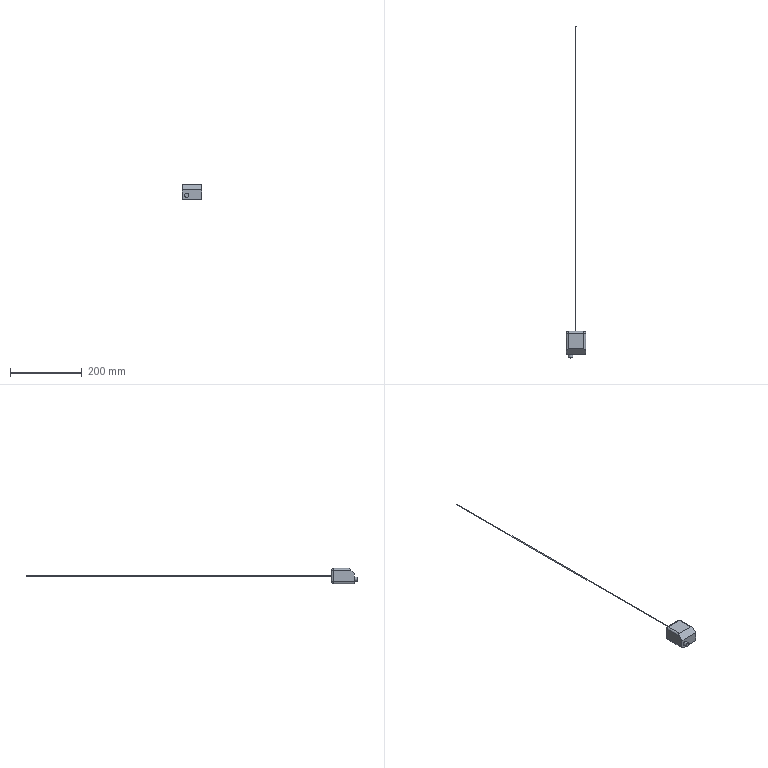Part | NX | 1 solid | 31 faces | box 54 x 924 x 42 mm | volume 140536 mm3 | cylinder 14 | plane 9 | cone 4 | sphere 4 | commonest cylinder face diameters 10 x8 2.5 x4 2 x1 12 x1
STEP:
#1=CARTESIAN_POINT('',(22.,64.,-16.));
#2=VERTEX_POINT('',#1);
#3=CARTESIAN_POINT('',(-22.,64.,-16.));
#4=VERTEX_POINT('',#3);
#5=CARTESIAN_POINT('',(0.,64.,-16.));
#6=DIRECTION('',(-1.,0.,0.));
#7=VECTOR('',#6,1000.);
#8=LINE('',#5,#7);
#9=EDGE_CURVE('',#2,#4,#8,.T.);
#10=ORIENTED_EDGE('',*,*,#9,.T.);
#11=CARTESIAN_POINT('',(-22.,64.,16.));
#12=VERTEX_POINT('',#11);
#13=CARTESIAN_POINT('',(-22.,64.,0.));
#14=DIRECTION('',(0.,0.,1.));
#15=VECTOR('',#14,1000.);
#16=LINE('',#13,#15);
#17=EDGE_CURVE('',#4,#12,#16,.T.);
#18=ORIENTED_EDGE('',*,*,#17,.T.);
#19=CARTESIAN_POINT('',(22.,64.,16.));
#20=VERTEX_POINT('',#19);
#21=CARTESIAN_POINT('',(0.,64.,16.));
#22=DIRECTION('',(1.,0.,0.));
#23=VECTOR('',#22,1000.);
#24=LINE('',#21,#23);
#25=EDGE_CURVE('',#12,#20,#24,.T.);
#26=ORIENTED_EDGE('',*,*,#25,.T.);
#27=CARTESIAN_POINT('',(22.,64.,0.));
#28=DIRECTION('',(0.,0.,-1.));
#29=VECTOR('',#28,1000.);
#30=LINE('',#27,#29);
#31=EDGE_CURVE('',#20,#2,#30,.T.);
#32=ORIENTED_EDGE('',*,*,#31,.T.);
#33=EDGE_LOOP('',(#10,#18,#26,#32));
#34=FACE_BOUND('',#33,.T.);
#35=CARTESIAN_POINT('',(0.,64.,-1.));
#36=VERTEX_POINT('',#35);
#37=CARTESIAN_POINT('',(0.,64.,0.));
#38=DIRECTION('',(0.,-1.,0.));
#39=DIRECTION('',(0.,0.,-1.));
#40=AXIS2_PLACEMENT_3D('',#37,#38,#39);
#41=CIRCLE('',#40,1.);
#42=EDGE_CURVE('',#36,#36,#41,.F.);
#43=ORIENTED_EDGE('',*,*,#42,.F.);
#44=EDGE_LOOP('',(#43));
#45=FACE_BOUND('',#44,.T.);
#46=CARTESIAN_POINT('',(0.,64.,0.));
#47=DIRECTION('',(0.,-1.,0.));
#48=DIRECTION('',(0.,0.,-1.));
#49=AXIS2_PLACEMENT_3D('',#46,#47,#48);
#50=PLANE('',#49);
#51=ADVANCED_FACE('',(#34,#45),#50,.F.);
#52=CARTESIAN_POINT('',(22.,0.,-21.));
#53=VERTEX_POINT('',#52);
#54=CARTESIAN_POINT('',(-22.,0.,-21.));
#55=VERTEX_POINT('',#54);
#56=CARTESIAN_POINT('',(-27.,0.,-21.));
#57=DIRECTION('',(-1.,0.,0.));
#58=VECTOR('',#57,1000.);
#59=LINE('',#56,#58);
#60=EDGE_CURVE('',#53,#55,#59,.T.);
#61=ORIENTED_EDGE('',*,*,#60,.F.);
#62=CARTESIAN_POINT('',(27.,0.,-16.));
#63=VERTEX_POINT('',#62);
#64=CARTESIAN_POINT('',(22.,0.,-16.));
#65=DIRECTION('',(0.,-1.,0.));
#66=DIRECTION('',(0.,0.,-1.));
#67=AXIS2_PLACEMENT_3D('',#64,#65,#66);
#68=CIRCLE('',#67,5.);
#69=EDGE_CURVE('',#53,#63,#68,.T.);
#70=ORIENTED_EDGE('',*,*,#69,.T.);
#71=CARTESIAN_POINT('',(27.,0.,6.));
#72=VERTEX_POINT('',#71);
#73=CARTESIAN_POINT('',(27.,0.,21.));
#74=DIRECTION('',(0.,0.,-1.));
#75=VECTOR('',#74,1000.);
#76=LINE('',#73,#75);
#77=EDGE_CURVE('',#72,#63,#76,.T.);
#78=ORIENTED_EDGE('',*,*,#77,.F.);
#79=CARTESIAN_POINT('',(-27.,0.,6.));
#80=VERTEX_POINT('',#79);
#81=CARTESIAN_POINT('',(-27.,0.,6.));
#82=DIRECTION('',(-1.,0.,0.));
#83=VECTOR('',#82,1000.);
#84=LINE('',#81,#83);
#85=EDGE_CURVE('',#72,#80,#84,.T.);
#86=ORIENTED_EDGE('',*,*,#85,.T.);
#87=CARTESIAN_POINT('',(-27.,0.,-16.));
#88=VERTEX_POINT('',#87);
#89=CARTESIAN_POINT('',(-27.,0.,21.));
#90=DIRECTION('',(0.,0.,1.));
#91=VECTOR('',#90,1000.);
#92=LINE('',#89,#91);
#93=EDGE_CURVE('',#88,#80,#92,.T.);
#94=ORIENTED_EDGE('',*,*,#93,.F.);
#95=CARTESIAN_POINT('',(-22.,0.,-16.));
#96=DIRECTION('',(0.,-1.,0.));
#97=DIRECTION('',(0.,0.,-1.));
#98=AXIS2_PLACEMENT_3D('',#95,#96,#97);
#99=CIRCLE('',#98,5.);
#100=EDGE_CURVE('',#88,#55,#99,.T.);
#101=ORIENTED_EDGE('',*,*,#100,.T.);
#102=EDGE_LOOP('',(#61,#70,#78,#86,#94,#101));
#103=FACE_BOUND('',#102,.T.);
#104=CARTESIAN_POINT('',(-15.,0.,-15.));
#105=VERTEX_POINT('',#104);
#106=CARTESIAN_POINT('',(-15.,0.,-9.));
#107=DIRECTION('',(0.,-1.,0.));
#108=DIRECTION('',(0.,0.,-1.));
#109=AXIS2_PLACEMENT_3D('',#106,#107,#108);
#110=CIRCLE('',#109,6.);
#111=EDGE_CURVE('',#105,#105,#110,.T.);
#112=ORIENTED_EDGE('',*,*,#111,.F.);
#113=EDGE_LOOP('',(#112));
#114=FACE_BOUND('',#113,.T.);
#115=CARTESIAN_POINT('',(0.,0.,0.));
#116=DIRECTION('',(0.,-1.,0.));
#117=DIRECTION('',(0.,0.,-1.));
#118=AXIS2_PLACEMENT_3D('',#115,#116,#117);
#119=PLANE('',#118);
#120=ADVANCED_FACE('',(#103,#114),#119,.T.);
#121=CARTESIAN_POINT('',(27.,59.,-16.));
#122=VERTEX_POINT('',#121);
#123=CARTESIAN_POINT('',(27.,64.,-16.));
#124=DIRECTION('',(0.,-1.,0.));
#125=VECTOR('',#124,1000.);
#126=LINE('',#123,#125);
#127=EDGE_CURVE('',#63,#122,#126,.F.);
#128=ORIENTED_EDGE('',*,*,#127,.T.);
#129=CARTESIAN_POINT('',(27.,59.,16.));
#130=VERTEX_POINT('',#129);
#131=CARTESIAN_POINT('',(27.,59.,21.));
#132=DIRECTION('',(0.,0.,-1.));
#133=VECTOR('',#132,1000.);
#134=LINE('',#131,#133);
#135=EDGE_CURVE('',#122,#130,#134,.F.);
#136=ORIENTED_EDGE('',*,*,#135,.T.);
#137=CARTESIAN_POINT('',(27.,10.,16.));
#138=VERTEX_POINT('',#137);
#139=CARTESIAN_POINT('',(27.,64.,16.));
#140=DIRECTION('',(0.,-1.,0.));
#141=VECTOR('',#140,1000.);
#142=LINE('',#139,#141);
#143=EDGE_CURVE('',#130,#138,#142,.T.);
#144=ORIENTED_EDGE('',*,*,#143,.T.);
#145=CARTESIAN_POINT('',(27.,15.,21.));
#146=DIRECTION('',(0.,-0.7071,-0.7071));
#147=VECTOR('',#146,1000.);
#148=LINE('',#145,#147);
#149=EDGE_CURVE('',#138,#72,#148,.T.);
#150=ORIENTED_EDGE('',*,*,#149,.T.);
#151=ORIENTED_EDGE('',*,*,#77,.T.);
#152=EDGE_LOOP('',(#128,#136,#144,#150,#151));
#153=FACE_BOUND('',#152,.T.);
#154=CARTESIAN_POINT('',(27.,64.,21.));
#155=DIRECTION('',(-1.,0.,0.));
#156=DIRECTION('',(0.,0.,1.));
#157=AXIS2_PLACEMENT_3D('',#154,#155,#156);
#158=PLANE('',#157);
#159=ADVANCED_FACE('',(#153),#158,.F.);
#160=CARTESIAN_POINT('',(17.25,46.4,-21.));
#161=VERTEX_POINT('',#160);
#162=CARTESIAN_POINT('',(18.5,46.4,-21.));
#163=DIRECTION('',(0.,0.,-1.));
#164=DIRECTION('',(-1.,0.,0.));
#165=AXIS2_PLACEMENT_3D('',#162,#163,#164);
#166=CIRCLE('',#165,1.25);
#167=EDGE_CURVE('',#161,#161,#166,.T.);
#168=ORIENTED_EDGE('',*,*,#167,.F.);
#169=EDGE_LOOP('',(#168));
#170=FACE_BOUND('',#169,.T.);
#171=CARTESIAN_POINT('',(-19.75,46.4,-21.));
#172=VERTEX_POINT('',#171);
#173=CARTESIAN_POINT('',(-18.5,46.4,-21.));
#174=DIRECTION('',(0.,0.,-1.));
#175=DIRECTION('',(-1.,0.,0.));
#176=AXIS2_PLACEMENT_3D('',#173,#174,#175);
#177=CIRCLE('',#176,1.25);
#178=EDGE_CURVE('',#172,#172,#177,.T.);
#179=ORIENTED_EDGE('',*,*,#178,.F.);
#180=EDGE_LOOP('',(#179));
#181=FACE_BOUND('',#180,.T.);
#182=CARTESIAN_POINT('',(17.25,26.4,-21.));
#183=VERTEX_POINT('',#182);
#184=CARTESIAN_POINT('',(18.5,26.4,-21.));
#185=DIRECTION('',(0.,0.,-1.));
#186=DIRECTION('',(-1.,0.,0.));
#187=AXIS2_PLACEMENT_3D('',#184,#185,#186);
#188=CIRCLE('',#187,1.25);
#189=EDGE_CURVE('',#183,#183,#188,.T.);
#190=ORIENTED_EDGE('',*,*,#189,.F.);
#191=EDGE_LOOP('',(#190));
#192=FACE_BOUND('',#191,.T.);
#193=CARTESIAN_POINT('',(-19.75,26.4,-21.));
#194=VERTEX_POINT('',#193);
#195=CARTESIAN_POINT('',(-18.5,26.4,-21.));
#196=DIRECTION('',(0.,0.,-1.));
#197=DIRECTION('',(-1.,0.,0.));
#198=AXIS2_PLACEMENT_3D('',#195,#196,#197);
#199=CIRCLE('',#198,1.25);
#200=EDGE_CURVE('',#194,#194,#199,.T.);
#201=ORIENTED_EDGE('',*,*,#200,.F.);
#202=EDGE_LOOP('',(#201));
#203=FACE_BOUND('',#202,.T.);
#204=CARTESIAN_POINT('',(-22.,59.,-21.));
#205=VERTEX_POINT('',#204);
#206=CARTESIAN_POINT('',(-22.,64.,-21.));
#207=DIRECTION('',(0.,-1.,0.));
#208=VECTOR('',#207,1000.);
#209=LINE('',#206,#208);
#210=EDGE_CURVE('',#55,#205,#209,.F.);
#211=ORIENTED_EDGE('',*,*,#210,.T.);
#212=CARTESIAN_POINT('',(22.,59.,-21.));
#213=VERTEX_POINT('',#212);
#214=CARTESIAN_POINT('',(-27.,59.,-21.));
#215=DIRECTION('',(-1.,0.,0.));
#216=VECTOR('',#215,1000.);
#217=LINE('',#214,#216);
#218=EDGE_CURVE('',#205,#213,#217,.F.);
#219=ORIENTED_EDGE('',*,*,#218,.T.);
#220=CARTESIAN_POINT('',(22.,64.,-21.));
#221=DIRECTION('',(0.,-1.,0.));
#222=VECTOR('',#221,1000.);
#223=LINE('',#220,#222);
#224=EDGE_CURVE('',#213,#53,#223,.T.);
#225=ORIENTED_EDGE('',*,*,#224,.T.);
#226=ORIENTED_EDGE('',*,*,#60,.T.);
#227=EDGE_LOOP('',(#211,#219,#225,#226));
#228=FACE_BOUND('',#227,.T.);
#229=CARTESIAN_POINT('',(-27.,64.,-21.));
#230=DIRECTION('',(0.,0.,1.));
#231=DIRECTION('',(1.,0.,0.));
#232=AXIS2_PLACEMENT_3D('',#229,#230,#231);
#233=PLANE('',#232);
#234=ADVANCED_FACE('',(#170,#181,#192,#203,#228),#233,.F.);
#235=CARTESIAN_POINT('',(-27.,10.,16.));
#236=VERTEX_POINT('',#235);
#237=CARTESIAN_POINT('',(-27.,59.,16.));
#238=VERTEX_POINT('',#237);
#239=CARTESIAN_POINT('',(-27.,64.,16.));
#240=DIRECTION('',(0.,-1.,0.));
#241=VECTOR('',#240,1000.);
#242=LINE('',#239,#241);
#243=EDGE_CURVE('',#236,#238,#242,.F.);
#244=ORIENTED_EDGE('',*,*,#243,.T.);
#245=CARTESIAN_POINT('',(-27.,59.,-16.));
#246=VERTEX_POINT('',#245);
#247=CARTESIAN_POINT('',(-27.,59.,21.));
#248=DIRECTION('',(0.,0.,1.));
#249=VECTOR('',#248,1000.);
#250=LINE('',#247,#249);
#251=EDGE_CURVE('',#238,#246,#250,.F.);
#252=ORIENTED_EDGE('',*,*,#251,.T.);
#253=CARTESIAN_POINT('',(-27.,64.,-16.));
#254=DIRECTION('',(0.,-1.,0.));
#255=VECTOR('',#254,1000.);
#256=LINE('',#253,#255);
#257=EDGE_CURVE('',#246,#88,#256,.T.);
#258=ORIENTED_EDGE('',*,*,#257,.T.);
#259=ORIENTED_EDGE('',*,*,#93,.T.);
#260=CARTESIAN_POINT('',(-27.,15.,21.));
#261=DIRECTION('',(0.,0.7071,0.7071));
#262=VECTOR('',#261,1000.);
#263=LINE('',#260,#262);
#264=EDGE_CURVE('',#80,#236,#263,.T.);
#265=ORIENTED_EDGE('',*,*,#264,.T.);
#266=EDGE_LOOP('',(#244,#252,#258,#259,#265));
#267=FACE_BOUND('',#266,.T.);
#268=CARTESIAN_POINT('',(-27.,64.,21.));
#269=DIRECTION('',(1.,0.,0.));
#270=DIRECTION('',(0.,0.,-1.));
#271=AXIS2_PLACEMENT_3D('',#268,#269,#270);
#272=PLANE('',#271);
#273=ADVANCED_FACE('',(#267),#272,.F.);
#274=CARTESIAN_POINT('',(22.,15.,21.));
#275=VERTEX_POINT('',#274);
#276=CARTESIAN_POINT('',(22.,59.,21.));
#277=VERTEX_POINT('',#276);
#278=CARTESIAN_POINT('',(22.,64.,21.));
#279=DIRECTION('',(0.,-1.,0.));
#280=VECTOR('',#279,1000.);
#281=LINE('',#278,#280);
#282=EDGE_CURVE('',#275,#277,#281,.F.);
#283=ORIENTED_EDGE('',*,*,#282,.T.);
#284=CARTESIAN_POINT('',(-22.,59.,21.));
#285=VERTEX_POINT('',#284);
#286=CARTESIAN_POINT('',(-27.,59.,21.));
#287=DIRECTION('',(1.,0.,0.));
#288=VECTOR('',#287,1000.);
#289=LINE('',#286,#288);
#290=EDGE_CURVE('',#277,#285,#289,.F.);
#291=ORIENTED_EDGE('',*,*,#290,.T.);
#292=CARTESIAN_POINT('',(-22.,15.,21.));
#293=VERTEX_POINT('',#292);
#294=CARTESIAN_POINT('',(-22.,64.,21.));
#295=DIRECTION('',(0.,-1.,0.));
#296=VECTOR('',#295,1000.);
#297=LINE('',#294,#296);
#298=EDGE_CURVE('',#285,#293,#297,.T.);
#299=ORIENTED_EDGE('',*,*,#298,.T.);
#300=CARTESIAN_POINT('',(27.,15.,21.));
#301=DIRECTION('',(1.,0.,0.));
#302=VECTOR('',#301,1000.);
#303=LINE('',#300,#302);
#304=EDGE_CURVE('',#293,#275,#303,.T.);
#305=ORIENTED_EDGE('',*,*,#304,.T.);
#306=EDGE_LOOP('',(#283,#291,#299,#305));
#307=FACE_BOUND('',#306,.T.);
#308=CARTESIAN_POINT('',(-27.,64.,21.));
#309=DIRECTION('',(0.,0.,-1.));
#310=DIRECTION('',(-1.,0.,0.));
#311=AXIS2_PLACEMENT_3D('',#308,#309,#310);
#312=PLANE('',#311);
#313=ADVANCED_FACE('',(#307),#312,.F.);
#314=ORIENTED_EDGE('',*,*,#149,.F.);
#315=CARTESIAN_POINT('',(22.,10.,16.));
#316=DIRECTION('',(0.,-0.7071,0.7071));
#317=DIRECTION('',(0.,-0.7071,-0.7071));
#318=AXIS2_PLACEMENT_3D('',#315,#316,#317);
#319=ELLIPSE('',#318,7.071,5.);
#320=EDGE_CURVE('',#138,#275,#319,.T.);
#321=ORIENTED_EDGE('',*,*,#320,.T.);
#322=ORIENTED_EDGE('',*,*,#304,.F.);
#323=CARTESIAN_POINT('',(-22.,10.,16.));
#324=DIRECTION('',(0.,-0.7071,0.7071));
#325=DIRECTION('',(0.,-0.7071,-0.7071));
#326=AXIS2_PLACEMENT_3D('',#323,#324,#325);
#327=ELLIPSE('',#326,7.071,5.);
#328=EDGE_CURVE('',#293,#236,#327,.T.);
#329=ORIENTED_EDGE('',*,*,#328,.T.);
#330=ORIENTED_EDGE('',*,*,#264,.F.);
#331=ORIENTED_EDGE('',*,*,#85,.F.);
#332=EDGE_LOOP('',(#314,#321,#322,#329,#330,#331));
#333=FACE_BOUND('',#332,.T.);
#334=CARTESIAN_POINT('',(-27.,15.,21.));
#335=DIRECTION('',(0.,-0.7071,0.7071));
#336=DIRECTION('',(-1.,0.,0.));
#337=AXIS2_PLACEMENT_3D('',#334,#335,#336);
#338=PLANE('',#337);
#339=ADVANCED_FACE('',(#333),#338,.T.);
#340=CARTESIAN_POINT('',(-18.5,26.4,-11.749));
#341=VERTEX_POINT('',#340);
#342=VERTEX_LOOP('',#341);
#343=FACE_BOUND('',#342,.T.);
#344=CARTESIAN_POINT('',(-19.75,26.4,-12.5));
#345=VERTEX_POINT('',#344);
#346=CARTESIAN_POINT('',(-18.5,26.4,-12.5));
#347=DIRECTION('',(0.,0.,-1.));
#348=DIRECTION('',(-1.,0.,0.));
#349=AXIS2_PLACEMENT_3D('',#346,#347,#348);
#350=CIRCLE('',#349,1.25);
#351=EDGE_CURVE('',#345,#345,#350,.T.);
#352=ORIENTED_EDGE('',*,*,#351,.T.);
#353=EDGE_LOOP('',(#352));
#354=FACE_BOUND('',#353,.T.);
#355=CARTESIAN_POINT('',(-18.5,26.4,-12.5));
#356=DIRECTION('',(0.,0.,-1.));
#357=DIRECTION('',(-1.,0.,0.));
#358=AXIS2_PLACEMENT_3D('',#355,#356,#357);
#359=CONICAL_SURFACE('',#358,1.25,1.03);
#360=ADVANCED_FACE('',(#343,#354),#359,.F.);
#361=ORIENTED_EDGE('',*,*,#351,.F.);
#362=EDGE_LOOP('',(#361));
#363=FACE_BOUND('',#362,.T.);
#364=ORIENTED_EDGE('',*,*,#200,.T.);
#365=EDGE_LOOP('',(#364));
#366=FACE_BOUND('',#365,.T.);
#367=CARTESIAN_POINT('',(-18.5,26.4,-21.));
#368=DIRECTION('',(0.,0.,-1.));
#369=DIRECTION('',(-1.,0.,0.));
#370=AXIS2_PLACEMENT_3D('',#367,#368,#369);
#371=CYLINDRICAL_SURFACE('',#370,1.25);
#372=ADVANCED_FACE('',(#363,#366),#371,.F.);
#373=CARTESIAN_POINT('',(18.5,26.4,-11.749));
#374=VERTEX_POINT('',#373);
#375=VERTEX_LOOP('',#374);
#376=FACE_BOUND('',#375,.T.);
#377=CARTESIAN_POINT('',(17.25,26.4,-12.5));
#378=VERTEX_POINT('',#377);
#379=CARTESIAN_POINT('',(18.5,26.4,-12.5));
#380=DIRECTION('',(0.,0.,-1.));
#381=DIRECTION('',(-1.,0.,0.));
#382=AXIS2_PLACEMENT_3D('',#379,#380,#381);
#383=CIRCLE('',#382,1.25);
#384=EDGE_CURVE('',#378,#378,#383,.T.);
#385=ORIENTED_EDGE('',*,*,#384,.T.);
#386=EDGE_LOOP('',(#385));
#387=FACE_BOUND('',#386,.T.);
#388=CARTESIAN_POINT('',(18.5,26.4,-12.5));
#389=DIRECTION('',(0.,0.,-1.));
#390=DIRECTION('',(-1.,0.,0.));
#391=AXIS2_PLACEMENT_3D('',#388,#389,#390);
#392=CONICAL_SURFACE('',#391,1.25,1.03);
#393=ADVANCED_FACE('',(#376,#387),#392,.F.);
#394=ORIENTED_EDGE('',*,*,#384,.F.);
#395=EDGE_LOOP('',(#394));
#396=FACE_BOUND('',#395,.T.);
#397=ORIENTED_EDGE('',*,*,#189,.T.);
#398=EDGE_LOOP('',(#397));
#399=FACE_BOUND('',#398,.T.);
#400=CARTESIAN_POINT('',(18.5,26.4,-21.));
#401=DIRECTION('',(0.,0.,-1.));
#402=DIRECTION('',(-1.,0.,0.));
#403=AXIS2_PLACEMENT_3D('',#400,#401,#402);
#404=CYLINDRICAL_SURFACE('',#403,1.25);
#405=ADVANCED_FACE('',(#396,#399),#404,.F.);
#406=CARTESIAN_POINT('',(-18.5,46.4,-11.749));
#407=VERTEX_POINT('',#406);
#408=VERTEX_LOOP('',#407);
#409=FACE_BOUND('',#408,.T.);
#410=CARTESIAN_POINT('',(-19.75,46.4,-12.5));
#411=VERTEX_POINT('',#410);
#412=CARTESIAN_POINT('',(-18.5,46.4,-12.5));
#413=DIRECTION('',(0.,0.,-1.));
#414=DIRECTION('',(-1.,0.,0.));
#415=AXIS2_PLACEMENT_3D('',#412,#413,#414);
#416=CIRCLE('',#415,1.25);
#417=EDGE_CURVE('',#411,#411,#416,.T.);
#418=ORIENTED_EDGE('',*,*,#417,.T.);
#419=EDGE_LOOP('',(#418));
#420=FACE_BOUND('',#419,.T.);
#421=CARTESIAN_POINT('',(-18.5,46.4,-12.5));
#422=DIRECTION('',(0.,0.,-1.));
#423=DIRECTION('',(-1.,0.,0.));
#424=AXIS2_PLACEMENT_3D('',#421,#422,#423);
#425=CONICAL_SURFACE('',#424,1.25,1.03);
#426=ADVANCED_FACE('',(#409,#420),#425,.F.);
#427=ORIENTED_EDGE('',*,*,#417,.F.);
#428=EDGE_LOOP('',(#427));
#429=FACE_BOUND('',#428,.T.);
#430=ORIENTED_EDGE('',*,*,#178,.T.);
#431=EDGE_LOOP('',(#430));
#432=FACE_BOUND('',#431,.T.);
#433=CARTESIAN_POINT('',(-18.5,46.4,-21.));
#434=DIRECTION('',(0.,0.,-1.));
#435=DIRECTION('',(-1.,0.,0.));
#436=AXIS2_PLACEMENT_3D('',#433,#434,#435);
#437=CYLINDRICAL_SURFACE('',#436,1.25);
#438=ADVANCED_FACE('',(#429,#432),#437,.F.);
#439=CARTESIAN_POINT('',(18.5,46.4,-11.749));
#440=VERTEX_POINT('',#439);
#441=VERTEX_LOOP('',#440);
#442=FACE_BOUND('',#441,.T.);
#443=CARTESIAN_POINT('',(17.25,46.4,-12.5));
#444=VERTEX_POINT('',#443);
#445=CARTESIAN_POINT('',(18.5,46.4,-12.5));
#446=DIRECTION('',(0.,0.,-1.));
#447=DIRECTION('',(-1.,0.,0.));
#448=AXIS2_PLACEMENT_3D('',#445,#446,#447);
#449=CIRCLE('',#448,1.25);
#450=EDGE_CURVE('',#444,#444,#449,.T.);
#451=ORIENTED_EDGE('',*,*,#450,.T.);
#452=EDGE_LOOP('',(#451));
#453=FACE_BOUND('',#452,.T.);
#454=CARTESIAN_POINT('',(18.5,46.4,-12.5));
#455=DIRECTION('',(0.,0.,-1.));
#456=DIRECTION('',(-1.,0.,0.));
#457=AXIS2_PLACEMENT_3D('',#454,#455,#456);
#458=CONICAL_SURFACE('',#457,1.25,1.03);
#459=ADVANCED_FACE('',(#442,#453),#458,.F.);
#460=ORIENTED_EDGE('',*,*,#450,.F.);
#461=EDGE_LOOP('',(#460));
#462=FACE_BOUND('',#461,.T.);
#463=ORIENTED_EDGE('',*,*,#167,.T.);
#464=EDGE_LOOP('',(#463));
#465=FACE_BOUND('',#464,.T.);
#466=CARTESIAN_POINT('',(18.5,46.4,-21.));
#467=DIRECTION('',(0.,0.,-1.));
#468=DIRECTION('',(-1.,0.,0.));
#469=AXIS2_PLACEMENT_3D('',#466,#467,#468);
#470=CYLINDRICAL_SURFACE('',#469,1.25);
#471=ADVANCED_FACE('',(#462,#465),#470,.F.);
#472=ORIENTED_EDGE('',*,*,#143,.F.);
#473=CARTESIAN_POINT('',(22.,59.,16.));
#474=DIRECTION('',(0.,-1.,0.));
#475=DIRECTION('',(0.,0.,-1.));
#476=AXIS2_PLACEMENT_3D('',#473,#474,#475);
#477=CIRCLE('',#476,5.);
#478=EDGE_CURVE('',#130,#277,#477,.T.);
#479=ORIENTED_EDGE('',*,*,#478,.T.);
#480=ORIENTED_EDGE('',*,*,#282,.F.);
#481=ORIENTED_EDGE('',*,*,#320,.F.);
#482=EDGE_LOOP('',(#472,#479,#480,#481));
#483=FACE_BOUND('',#482,.T.);
#484=CARTESIAN_POINT('',(22.,64.,16.));
#485=DIRECTION('',(0.,-1.,0.));
#486=DIRECTION('',(0.,0.,-1.));
#487=AXIS2_PLACEMENT_3D('',#484,#485,#486);
#488=CYLINDRICAL_SURFACE('',#487,5.);
#489=ADVANCED_FACE('',(#483),#488,.T.);
#490=ORIENTED_EDGE('',*,*,#298,.F.);
#491=CARTESIAN_POINT('',(-22.,59.,16.));
#492=DIRECTION('',(0.,-1.,0.));
#493=DIRECTION('',(0.,0.,-1.));
#494=AXIS2_PLACEMENT_3D('',#491,#492,#493);
#495=CIRCLE('',#494,5.);
#496=EDGE_CURVE('',#285,#238,#495,.T.);
#497=ORIENTED_EDGE('',*,*,#496,.T.);
#498=ORIENTED_EDGE('',*,*,#243,.F.);
#499=ORIENTED_EDGE('',*,*,#328,.F.);
#500=EDGE_LOOP('',(#490,#497,#498,#499));
#501=FACE_BOUND('',#500,.T.);
#502=CARTESIAN_POINT('',(-22.,64.,16.));
#503=DIRECTION('',(0.,-1.,0.));
#504=DIRECTION('',(0.,0.,-1.));
#505=AXIS2_PLACEMENT_3D('',#502,#503,#504);
#506=CYLINDRICAL_SURFACE('',#505,5.);
#507=ADVANCED_FACE('',(#501),#506,.T.);
#508=ORIENTED_EDGE('',*,*,#224,.F.);
#509=CARTESIAN_POINT('',(22.,59.,-16.));
#510=DIRECTION('',(0.,-1.,0.));
#511=DIRECTION('',(0.,0.,-1.));
#512=AXIS2_PLACEMENT_3D('',#509,#510,#511);
#513=CIRCLE('',#512,5.);
#514=EDGE_CURVE('',#213,#122,#513,.T.);
#515=ORIENTED_EDGE('',*,*,#514,.T.);
#516=ORIENTED_EDGE('',*,*,#127,.F.);
#517=ORIENTED_EDGE('',*,*,#69,.F.);
#518=EDGE_LOOP('',(#508,#515,#516,#517));
#519=FACE_BOUND('',#518,.T.);
#520=CARTESIAN_POINT('',(22.,64.,-16.));
#521=DIRECTION('',(0.,-1.,0.));
#522=DIRECTION('',(0.,0.,-1.));
#523=AXIS2_PLACEMENT_3D('',#520,#521,#522);
#524=CYLINDRICAL_SURFACE('',#523,5.);
#525=ADVANCED_FACE('',(#519),#524,.T.);
#526=ORIENTED_EDGE('',*,*,#257,.F.);
#527=CARTESIAN_POINT('',(-22.,59.,-16.));
#528=DIRECTION('',(0.,-1.,0.));
#529=DIRECTION('',(0.,0.,-1.));
#530=AXIS2_PLACEMENT_3D('',#527,#528,#529);
#531=CIRCLE('',#530,5.);
#532=EDGE_CURVE('',#246,#205,#531,.T.);
#533=ORIENTED_EDGE('',*,*,#532,.T.);
#534=ORIENTED_EDGE('',*,*,#210,.F.);
#535=ORIENTED_EDGE('',*,*,#100,.F.);
#536=EDGE_LOOP('',(#526,#533,#534,#535));
#537=FACE_BOUND('',#536,.T.);
#538=CARTESIAN_POINT('',(-22.,64.,-16.));
#539=DIRECTION('',(0.,-1.,0.));
#540=DIRECTION('',(0.,0.,-1.));
#541=AXIS2_PLACEMENT_3D('',#538,#539,#540);
#542=CYLINDRICAL_SURFACE('',#541,5.);
#543=ADVANCED_FACE('',(#537),#542,.T.);
#544=CARTESIAN_POINT('',(-15.,-10.,-15.));
#545=VERTEX_POINT('',#544);
#546=CARTESIAN_POINT('',(-15.,-10.,-9.));
#547=DIRECTION('',(0.,-1.,0.));
#548=DIRECTION('',(0.,0.,-1.));
#549=AXIS2_PLACEMENT_3D('',#546,#547,#548);
#550=CIRCLE('',#549,6.);
#551=EDGE_CURVE('',#545,#545,#550,.T.);
#552=ORIENTED_EDGE('',*,*,#551,.F.);
#553=EDGE_LOOP('',(#552));
#554=FACE_BOUND('',#553,.T.);
#555=ORIENTED_EDGE('',*,*,#111,.T.);
#556=EDGE_LOOP('',(#555));
#557=FACE_BOUND('',#556,.T.);
#558=CARTESIAN_POINT('',(-15.,-10.,-9.));
#559=DIRECTION('',(0.,1.,0.));
#560=DIRECTION('',(0.,0.,1.));
#561=AXIS2_PLACEMENT_3D('',#558,#559,#560);
#562=CYLINDRICAL_SURFACE('',#561,6.);
#563=ADVANCED_FACE('',(#554,#557),#562,.T.);
#564=ORIENTED_EDGE('',*,*,#551,.T.);
#565=EDGE_LOOP('',(#564));
#566=FACE_BOUND('',#565,.T.);
#567=CARTESIAN_POINT('',(-15.,-10.,-9.));
#568=DIRECTION('',(0.,-1.,0.));
#569=DIRECTION('',(0.,0.,-1.));
#570=AXIS2_PLACEMENT_3D('',#567,#568,#569);
#571=PLANE('',#570);
#572=ADVANCED_FACE('',(#566),#571,.T.);
#573=CARTESIAN_POINT('',(22.,59.,-16.));
#574=DIRECTION('',(0.,0.,1.));
#575=DIRECTION('',(1.,0.,0.));
#576=AXIS2_PLACEMENT_3D('',#573,#574,#575);
#577=CIRCLE('',#576,5.);
#578=EDGE_CURVE('',#122,#2,#577,.T.);
#579=ORIENTED_EDGE('',*,*,#578,.F.);
#580=ORIENTED_EDGE('',*,*,#514,.F.);
#581=CARTESIAN_POINT('',(22.,59.,-16.));
#582=DIRECTION('',(-1.,0.,0.));
#583=DIRECTION('',(0.,0.,1.));
#584=AXIS2_PLACEMENT_3D('',#581,#582,#583);
#585=CIRCLE('',#584,5.);
#586=EDGE_CURVE('',#2,#213,#585,.T.);
#587=ORIENTED_EDGE('',*,*,#586,.F.);
#588=EDGE_LOOP('',(#579,#580,#587));
#589=FACE_BOUND('',#588,.T.);
#590=CARTESIAN_POINT('',(22.,59.,-16.));
#591=DIRECTION('',(0.,0.,1.));
#592=DIRECTION('',(1.,0.,0.));
#593=AXIS2_PLACEMENT_3D('',#590,#591,#592);
#594=SPHERICAL_SURFACE('',#593,5.);
#595=ADVANCED_FACE('',(#589),#594,.T.);
#596=ORIENTED_EDGE('',*,*,#586,.T.);
#597=ORIENTED_EDGE('',*,*,#218,.F.);
#598=CARTESIAN_POINT('',(-22.,59.,-16.));
#599=DIRECTION('',(-1.,0.,0.));
#600=DIRECTION('',(0.,0.,1.));
#601=AXIS2_PLACEMENT_3D('',#598,#599,#600);
#602=CIRCLE('',#601,5.);
#603=EDGE_CURVE('',#4,#205,#602,.T.);
#604=ORIENTED_EDGE('',*,*,#603,.F.);
#605=ORIENTED_EDGE('',*,*,#9,.F.);
#606=EDGE_LOOP('',(#596,#597,#604,#605));
#607=FACE_BOUND('',#606,.T.);
#608=CARTESIAN_POINT('',(0.,59.,-16.));
#609=DIRECTION('',(-1.,0.,0.));
#610=DIRECTION('',(0.,0.,1.));
#611=AXIS2_PLACEMENT_3D('',#608,#609,#610);
#612=CYLINDRICAL_SURFACE('',#611,5.);
#613=ADVANCED_FACE('',(#607),#612,.T.);
#614=ORIENTED_EDGE('',*,*,#578,.T.);
#615=ORIENTED_EDGE('',*,*,#31,.F.);
#616=CARTESIAN_POINT('',(22.,59.,16.));
#617=DIRECTION('',(0.,0.,1.));
#618=DIRECTION('',(1.,0.,0.));
#619=AXIS2_PLACEMENT_3D('',#616,#617,#618);
#620=CIRCLE('',#619,5.);
#621=EDGE_CURVE('',#130,#20,#620,.T.);
#622=ORIENTED_EDGE('',*,*,#621,.F.);
#623=ORIENTED_EDGE('',*,*,#135,.F.);
#624=EDGE_LOOP('',(#614,#615,#622,#623));
#625=FACE_BOUND('',#624,.T.);
#626=CARTESIAN_POINT('',(22.,59.,0.));
#627=DIRECTION('',(0.,0.,-1.));
#628=DIRECTION('',(-1.,0.,0.));
#629=AXIS2_PLACEMENT_3D('',#626,#627,#628);
#630=CYLINDRICAL_SURFACE('',#629,5.);
#631=ADVANCED_FACE('',(#625),#630,.T.);
#632=ORIENTED_EDGE('',*,*,#603,.T.);
#633=ORIENTED_EDGE('',*,*,#532,.F.);
#634=CARTESIAN_POINT('',(-22.,59.,-16.));
#635=DIRECTION('',(0.,0.,1.));
#636=DIRECTION('',(1.,0.,0.));
#637=AXIS2_PLACEMENT_3D('',#634,#635,#636);
#638=CIRCLE('',#637,5.);
#639=EDGE_CURVE('',#4,#246,#638,.T.);
#640=ORIENTED_EDGE('',*,*,#639,.F.);
#641=EDGE_LOOP('',(#632,#633,#640));
#642=FACE_BOUND('',#641,.T.);
#643=CARTESIAN_POINT('',(-22.,59.,-16.));
#644=DIRECTION('',(0.,0.,1.));
#645=DIRECTION('',(1.,0.,0.));
#646=AXIS2_PLACEMENT_3D('',#643,#644,#645);
#647=SPHERICAL_SURFACE('',#646,5.);
#648=ADVANCED_FACE('',(#642),#647,.T.);
#649=ORIENTED_EDGE('',*,*,#478,.F.);
#650=ORIENTED_EDGE('',*,*,#621,.T.);
#651=CARTESIAN_POINT('',(22.,59.,16.));
#652=DIRECTION('',(-1.,0.,0.));
#653=DIRECTION('',(0.,0.,1.));
#654=AXIS2_PLACEMENT_3D('',#651,#652,#653);
#655=CIRCLE('',#654,5.);
#656=EDGE_CURVE('',#277,#20,#655,.T.);
#657=ORIENTED_EDGE('',*,*,#656,.F.);
#658=EDGE_LOOP('',(#649,#650,#657));
#659=FACE_BOUND('',#658,.T.);
#660=CARTESIAN_POINT('',(22.,59.,16.));
#661=DIRECTION('',(0.,0.,1.));
#662=DIRECTION('',(1.,0.,0.));
#663=AXIS2_PLACEMENT_3D('',#660,#661,#662);
#664=SPHERICAL_SURFACE('',#663,5.);
#665=ADVANCED_FACE('',(#659),#664,.T.);
#666=ORIENTED_EDGE('',*,*,#639,.T.);
#667=ORIENTED_EDGE('',*,*,#251,.F.);
#668=CARTESIAN_POINT('',(-22.,59.,16.));
#669=DIRECTION('',(0.,0.,1.));
#670=DIRECTION('',(1.,0.,0.));
#671=AXIS2_PLACEMENT_3D('',#668,#669,#670);
#672=CIRCLE('',#671,5.);
#673=EDGE_CURVE('',#12,#238,#672,.T.);
#674=ORIENTED_EDGE('',*,*,#673,.F.);
#675=ORIENTED_EDGE('',*,*,#17,.F.);
#676=EDGE_LOOP('',(#666,#667,#674,#675));
#677=FACE_BOUND('',#676,.T.);
#678=CARTESIAN_POINT('',(-22.,59.,0.));
#679=DIRECTION('',(0.,0.,1.));
#680=DIRECTION('',(1.,0.,0.));
#681=AXIS2_PLACEMENT_3D('',#678,#679,#680);
#682=CYLINDRICAL_SURFACE('',#681,5.);
#683=ADVANCED_FACE('',(#677),#682,.T.);
#684=ORIENTED_EDGE('',*,*,#656,.T.);
#685=ORIENTED_EDGE('',*,*,#25,.F.);
#686=CARTESIAN_POINT('',(-22.,59.,16.));
#687=DIRECTION('',(-1.,0.,0.));
#688=DIRECTION('',(0.,0.,1.));
#689=AXIS2_PLACEMENT_3D('',#686,#687,#688);
#690=CIRCLE('',#689,5.);
#691=EDGE_CURVE('',#285,#12,#690,.T.);
#692=ORIENTED_EDGE('',*,*,#691,.F.);
#693=ORIENTED_EDGE('',*,*,#290,.F.);
#694=EDGE_LOOP('',(#684,#685,#692,#693));
#695=FACE_BOUND('',#694,.T.);
#696=CARTESIAN_POINT('',(0.,59.,16.));
#697=DIRECTION('',(1.,0.,0.));
#698=DIRECTION('',(0.,0.,-1.));
#699=AXIS2_PLACEMENT_3D('',#696,#697,#698);
#700=CYLINDRICAL_SURFACE('',#699,5.);
#701=ADVANCED_FACE('',(#695),#700,.T.);
#702=ORIENTED_EDGE('',*,*,#673,.T.);
#703=ORIENTED_EDGE('',*,*,#496,.F.);
#704=ORIENTED_EDGE('',*,*,#691,.T.);
#705=EDGE_LOOP('',(#702,#703,#704));
#706=FACE_BOUND('',#705,.T.);
#707=CARTESIAN_POINT('',(-22.,59.,16.));
#708=DIRECTION('',(0.,0.,1.));
#709=DIRECTION('',(1.,0.,0.));
#710=AXIS2_PLACEMENT_3D('',#707,#708,#709);
#711=SPHERICAL_SURFACE('',#710,5.);
#712=ADVANCED_FACE('',(#706),#711,.T.);
#713=CARTESIAN_POINT('',(0.,914.,1.));
#714=VERTEX_POINT('',#713);
#715=CARTESIAN_POINT('',(0.,914.,0.));
#716=DIRECTION('',(0.,1.,0.));
#717=DIRECTION('',(0.,0.,1.));
#718=AXIS2_PLACEMENT_3D('',#715,#716,#717);
#719=CIRCLE('',#718,1.);
#720=EDGE_CURVE('',#714,#714,#719,.T.);
#721=ORIENTED_EDGE('',*,*,#720,.F.);
#722=EDGE_LOOP('',(#721));
#723=FACE_BOUND('',#722,.T.);
#724=ORIENTED_EDGE('',*,*,#42,.T.);
#725=EDGE_LOOP('',(#724));
#726=FACE_BOUND('',#725,.T.);
#727=CARTESIAN_POINT('',(0.,914.,0.));
#728=DIRECTION('',(0.,-1.,0.));
#729=DIRECTION('',(0.,0.,-1.));
#730=AXIS2_PLACEMENT_3D('',#727,#728,#729);
#731=CYLINDRICAL_SURFACE('',#730,1.);
#732=ADVANCED_FACE('',(#723,#726),#731,.T.);
#733=ORIENTED_EDGE('',*,*,#720,.T.);
#734=EDGE_LOOP('',(#733));
#735=FACE_BOUND('',#734,.T.);
#736=CARTESIAN_POINT('',(0.,914.,0.));
#737=DIRECTION('',(0.,1.,0.));
#738=DIRECTION('',(0.,0.,1.));
#739=AXIS2_PLACEMENT_3D('',#736,#737,#738);
#740=PLANE('',#739);
#741=ADVANCED_FACE('',(#735),#740,.T.);
#742=CLOSED_SHELL('',(#51,#120,#159,#234,#273,#313,#339,#360,#372,#393,#405,#426,#438,#459,#471,#489,#507,#525,#543,#563,#572,#595,#613,#631,#648,#665,#683,#701,#712,#732,#741));
#743=MANIFOLD_SOLID_BREP('',#742);
#744=(LENGTH_UNIT()NAMED_UNIT(*)SI_UNIT(.MILLI.,.METRE.));
#745=UNCERTAINTY_MEASURE_WITH_UNIT(LENGTH_MEASURE(0.00001),#744,'','');
#746=(NAMED_UNIT(*)PLANE_ANGLE_UNIT()SI_UNIT($,.RADIAN.));
#747=(NAMED_UNIT(*)SI_UNIT($,.STERADIAN.)SOLID_ANGLE_UNIT());
#748=(GEOMETRIC_REPRESENTATION_CONTEXT(3)GLOBAL_UNCERTAINTY_ASSIGNED_CONTEXT((#745))GLOBAL_UNIT_ASSIGNED_CONTEXT((#744,#746,#747))REPRESENTATION_CONTEXT('',''));
#749=ADVANCED_BREP_SHAPE_REPRESENTATION('',(#743),#748);